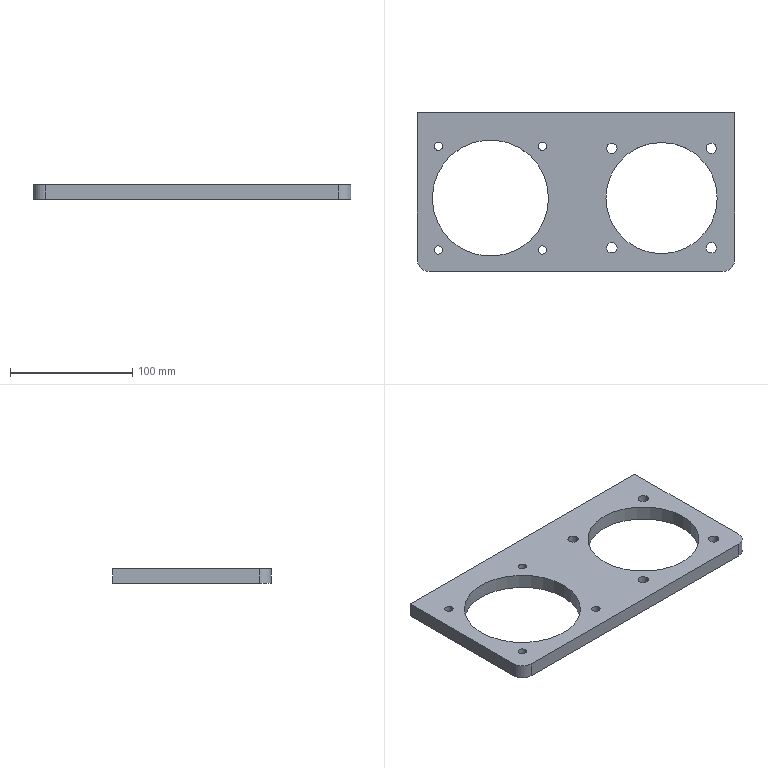Part | SolidWorks | features HoleWzd 2, FlatPattern 1, SMBaseFlange 1, SheetMetal 1 | 1 solid | 28 faces | box 260 x 130 x 12 mm | volume 237513 mm3 | cylinder 22 | plane 6 | commonest cylinder face diameters 6.8 x8 8.5 x8 20 x2 91 x2 95 x2
STEP:
#1=CARTESIAN_POINT('',(25.1,35.65,-12.));
#2=VERTEX_POINT('',#1);
#3=CARTESIAN_POINT('',(33.6,35.65,-12.));
#4=VERTEX_POINT('',#3);
#5=CARTESIAN_POINT('',(29.35,35.65,-12.));
#6=DIRECTION('',(0.,0.,1.));
#7=DIRECTION('',(1.,0.,0.));
#8=AXIS2_PLACEMENT_3D('',#5,#6,#7);
#9=CIRCLE('',#8,4.25);
#10=EDGE_CURVE('',#2,#4,#9,.T.);
#11=ORIENTED_EDGE('',*,*,#10,.F.);
#12=CARTESIAN_POINT('',(25.1,35.65,0.));
#13=VERTEX_POINT('',#12);
#14=CARTESIAN_POINT('',(25.1,35.65,0.));
#15=DIRECTION('',(0.,0.,1.));
#16=VECTOR('',#15,1000.);
#17=LINE('',#14,#16);
#18=EDGE_CURVE('',#2,#13,#17,.T.);
#19=ORIENTED_EDGE('',*,*,#18,.T.);
#20=CARTESIAN_POINT('',(33.6,35.65,0.));
#21=VERTEX_POINT('',#20);
#22=CARTESIAN_POINT('',(29.35,35.65,0.));
#23=DIRECTION('',(0.,0.,1.));
#24=DIRECTION('',(1.,0.,0.));
#25=AXIS2_PLACEMENT_3D('',#22,#23,#24);
#26=CIRCLE('',#25,4.25);
#27=EDGE_CURVE('',#13,#21,#26,.T.);
#28=ORIENTED_EDGE('',*,*,#27,.T.);
#29=CARTESIAN_POINT('',(33.6,35.65,0.));
#30=DIRECTION('',(0.,0.,1.));
#31=VECTOR('',#30,1000.);
#32=LINE('',#29,#31);
#33=EDGE_CURVE('',#4,#21,#32,.T.);
#34=ORIENTED_EDGE('',*,*,#33,.F.);
#35=EDGE_LOOP('',(#11,#19,#28,#34));
#36=FACE_OUTER_BOUND('',#35,.T.);
#37=CARTESIAN_POINT('',(29.35,35.65,0.));
#38=DIRECTION('',(0.,0.,1.));
#39=DIRECTION('',(1.,0.,0.));
#40=AXIS2_PLACEMENT_3D('',#37,#38,#39);
#41=CYLINDRICAL_SURFACE('',#40,4.25);
#42=ADVANCED_FACE('',(#36),#41,.F.);
#43=CARTESIAN_POINT('',(106.4,35.65,-12.));
#44=VERTEX_POINT('',#43);
#45=CARTESIAN_POINT('',(114.9,35.65,-12.));
#46=VERTEX_POINT('',#45);
#47=CARTESIAN_POINT('',(110.65,35.65,-12.));
#48=DIRECTION('',(0.,0.,1.));
#49=DIRECTION('',(1.,0.,0.));
#50=AXIS2_PLACEMENT_3D('',#47,#48,#49);
#51=CIRCLE('',#50,4.25);
#52=EDGE_CURVE('',#44,#46,#51,.T.);
#53=ORIENTED_EDGE('',*,*,#52,.F.);
#54=CARTESIAN_POINT('',(106.4,35.65,0.));
#55=VERTEX_POINT('',#54);
#56=CARTESIAN_POINT('',(106.4,35.65,0.));
#57=DIRECTION('',(0.,0.,1.));
#58=VECTOR('',#57,1000.);
#59=LINE('',#56,#58);
#60=EDGE_CURVE('',#44,#55,#59,.T.);
#61=ORIENTED_EDGE('',*,*,#60,.T.);
#62=CARTESIAN_POINT('',(114.9,35.65,0.));
#63=VERTEX_POINT('',#62);
#64=CARTESIAN_POINT('',(110.65,35.65,0.));
#65=DIRECTION('',(0.,0.,1.));
#66=DIRECTION('',(1.,0.,0.));
#67=AXIS2_PLACEMENT_3D('',#64,#65,#66);
#68=CIRCLE('',#67,4.25);
#69=EDGE_CURVE('',#55,#63,#68,.T.);
#70=ORIENTED_EDGE('',*,*,#69,.T.);
#71=CARTESIAN_POINT('',(114.9,35.65,0.));
#72=DIRECTION('',(0.,0.,1.));
#73=VECTOR('',#72,1000.);
#74=LINE('',#71,#73);
#75=EDGE_CURVE('',#46,#63,#74,.T.);
#76=ORIENTED_EDGE('',*,*,#75,.F.);
#77=EDGE_LOOP('',(#53,#61,#70,#76));
#78=FACE_OUTER_BOUND('',#77,.T.);
#79=CARTESIAN_POINT('',(110.65,35.65,0.));
#80=DIRECTION('',(0.,0.,1.));
#81=DIRECTION('',(1.,0.,0.));
#82=AXIS2_PLACEMENT_3D('',#79,#80,#81);
#83=CYLINDRICAL_SURFACE('',#82,4.25);
#84=ADVANCED_FACE('',(#78),#83,.F.);
#85=CARTESIAN_POINT('',(106.4,-45.65,-12.));
#86=VERTEX_POINT('',#85);
#87=CARTESIAN_POINT('',(114.9,-45.65,-12.));
#88=VERTEX_POINT('',#87);
#89=CARTESIAN_POINT('',(110.65,-45.65,-12.));
#90=DIRECTION('',(0.,0.,1.));
#91=DIRECTION('',(1.,0.,0.));
#92=AXIS2_PLACEMENT_3D('',#89,#90,#91);
#93=CIRCLE('',#92,4.25);
#94=EDGE_CURVE('',#86,#88,#93,.T.);
#95=ORIENTED_EDGE('',*,*,#94,.F.);
#96=CARTESIAN_POINT('',(106.4,-45.65,0.));
#97=VERTEX_POINT('',#96);
#98=CARTESIAN_POINT('',(106.4,-45.65,0.));
#99=DIRECTION('',(0.,0.,1.));
#100=VECTOR('',#99,1000.);
#101=LINE('',#98,#100);
#102=EDGE_CURVE('',#86,#97,#101,.T.);
#103=ORIENTED_EDGE('',*,*,#102,.T.);
#104=CARTESIAN_POINT('',(114.9,-45.65,0.));
#105=VERTEX_POINT('',#104);
#106=CARTESIAN_POINT('',(110.65,-45.65,0.));
#107=DIRECTION('',(0.,0.,1.));
#108=DIRECTION('',(1.,0.,0.));
#109=AXIS2_PLACEMENT_3D('',#106,#107,#108);
#110=CIRCLE('',#109,4.25);
#111=EDGE_CURVE('',#97,#105,#110,.T.);
#112=ORIENTED_EDGE('',*,*,#111,.T.);
#113=CARTESIAN_POINT('',(114.9,-45.65,0.));
#114=DIRECTION('',(0.,0.,1.));
#115=VECTOR('',#114,1000.);
#116=LINE('',#113,#115);
#117=EDGE_CURVE('',#88,#105,#116,.T.);
#118=ORIENTED_EDGE('',*,*,#117,.F.);
#119=EDGE_LOOP('',(#95,#103,#112,#118));
#120=FACE_OUTER_BOUND('',#119,.T.);
#121=CARTESIAN_POINT('',(110.65,-45.65,0.));
#122=DIRECTION('',(0.,0.,1.));
#123=DIRECTION('',(1.,0.,0.));
#124=AXIS2_PLACEMENT_3D('',#121,#122,#123);
#125=CYLINDRICAL_SURFACE('',#124,4.25);
#126=ADVANCED_FACE('',(#120),#125,.F.);
#127=CARTESIAN_POINT('',(25.1,-45.65,-12.));
#128=VERTEX_POINT('',#127);
#129=CARTESIAN_POINT('',(33.6,-45.65,-12.));
#130=VERTEX_POINT('',#129);
#131=CARTESIAN_POINT('',(29.35,-45.65,-12.));
#132=DIRECTION('',(0.,0.,1.));
#133=DIRECTION('',(1.,0.,0.));
#134=AXIS2_PLACEMENT_3D('',#131,#132,#133);
#135=CIRCLE('',#134,4.25);
#136=EDGE_CURVE('',#128,#130,#135,.T.);
#137=ORIENTED_EDGE('',*,*,#136,.F.);
#138=CARTESIAN_POINT('',(25.1,-45.65,0.));
#139=VERTEX_POINT('',#138);
#140=CARTESIAN_POINT('',(25.1,-45.65,0.));
#141=DIRECTION('',(0.,0.,1.));
#142=VECTOR('',#141,1000.);
#143=LINE('',#140,#142);
#144=EDGE_CURVE('',#128,#139,#143,.T.);
#145=ORIENTED_EDGE('',*,*,#144,.T.);
#146=CARTESIAN_POINT('',(33.6,-45.65,0.));
#147=VERTEX_POINT('',#146);
#148=CARTESIAN_POINT('',(29.35,-45.65,0.));
#149=DIRECTION('',(0.,0.,1.));
#150=DIRECTION('',(1.,0.,0.));
#151=AXIS2_PLACEMENT_3D('',#148,#149,#150);
#152=CIRCLE('',#151,4.25);
#153=EDGE_CURVE('',#139,#147,#152,.T.);
#154=ORIENTED_EDGE('',*,*,#153,.T.);
#155=CARTESIAN_POINT('',(33.6,-45.65,0.));
#156=DIRECTION('',(0.,0.,1.));
#157=VECTOR('',#156,1000.);
#158=LINE('',#155,#157);
#159=EDGE_CURVE('',#130,#147,#158,.T.);
#160=ORIENTED_EDGE('',*,*,#159,.F.);
#161=EDGE_LOOP('',(#137,#145,#154,#160));
#162=FACE_OUTER_BOUND('',#161,.T.);
#163=CARTESIAN_POINT('',(29.35,-45.65,0.));
#164=DIRECTION('',(0.,0.,1.));
#165=DIRECTION('',(1.,0.,0.));
#166=AXIS2_PLACEMENT_3D('',#163,#164,#165);
#167=CYLINDRICAL_SURFACE('',#166,4.25);
#168=ADVANCED_FACE('',(#162),#167,.F.);
#169=CARTESIAN_POINT('',(-115.9,37.5,-12.));
#170=VERTEX_POINT('',#169);
#171=CARTESIAN_POINT('',(-109.1,37.5,-12.));
#172=VERTEX_POINT('',#171);
#173=CARTESIAN_POINT('',(-112.5,37.5,-12.));
#174=DIRECTION('',(0.,0.,1.));
#175=DIRECTION('',(1.,0.,0.));
#176=AXIS2_PLACEMENT_3D('',#173,#174,#175);
#177=CIRCLE('',#176,3.4);
#178=EDGE_CURVE('',#170,#172,#177,.T.);
#179=ORIENTED_EDGE('',*,*,#178,.F.);
#180=CARTESIAN_POINT('',(-115.9,37.5,0.));
#181=VERTEX_POINT('',#180);
#182=CARTESIAN_POINT('',(-115.9,37.5,0.));
#183=DIRECTION('',(0.,0.,1.));
#184=VECTOR('',#183,1000.);
#185=LINE('',#182,#184);
#186=EDGE_CURVE('',#170,#181,#185,.T.);
#187=ORIENTED_EDGE('',*,*,#186,.T.);
#188=CARTESIAN_POINT('',(-109.1,37.5,0.));
#189=VERTEX_POINT('',#188);
#190=CARTESIAN_POINT('',(-112.5,37.5,0.));
#191=DIRECTION('',(0.,0.,1.));
#192=DIRECTION('',(1.,0.,0.));
#193=AXIS2_PLACEMENT_3D('',#190,#191,#192);
#194=CIRCLE('',#193,3.4);
#195=EDGE_CURVE('',#181,#189,#194,.T.);
#196=ORIENTED_EDGE('',*,*,#195,.T.);
#197=CARTESIAN_POINT('',(-109.1,37.5,0.));
#198=DIRECTION('',(0.,0.,1.));
#199=VECTOR('',#198,1000.);
#200=LINE('',#197,#199);
#201=EDGE_CURVE('',#172,#189,#200,.T.);
#202=ORIENTED_EDGE('',*,*,#201,.F.);
#203=EDGE_LOOP('',(#179,#187,#196,#202));
#204=FACE_OUTER_BOUND('',#203,.T.);
#205=CARTESIAN_POINT('',(-112.5,37.5,0.));
#206=DIRECTION('',(0.,0.,1.));
#207=DIRECTION('',(1.,0.,0.));
#208=AXIS2_PLACEMENT_3D('',#205,#206,#207);
#209=CYLINDRICAL_SURFACE('',#208,3.4);
#210=ADVANCED_FACE('',(#204),#209,.F.);
#211=CARTESIAN_POINT('',(-30.9,37.5,-12.));
#212=VERTEX_POINT('',#211);
#213=CARTESIAN_POINT('',(-24.1,37.5,-12.));
#214=VERTEX_POINT('',#213);
#215=CARTESIAN_POINT('',(-27.5,37.5,-12.));
#216=DIRECTION('',(0.,0.,1.));
#217=DIRECTION('',(1.,0.,0.));
#218=AXIS2_PLACEMENT_3D('',#215,#216,#217);
#219=CIRCLE('',#218,3.4);
#220=EDGE_CURVE('',#212,#214,#219,.T.);
#221=ORIENTED_EDGE('',*,*,#220,.F.);
#222=CARTESIAN_POINT('',(-30.9,37.5,0.));
#223=VERTEX_POINT('',#222);
#224=CARTESIAN_POINT('',(-30.9,37.5,0.));
#225=DIRECTION('',(0.,0.,1.));
#226=VECTOR('',#225,1000.);
#227=LINE('',#224,#226);
#228=EDGE_CURVE('',#212,#223,#227,.T.);
#229=ORIENTED_EDGE('',*,*,#228,.T.);
#230=CARTESIAN_POINT('',(-24.1,37.5,0.));
#231=VERTEX_POINT('',#230);
#232=CARTESIAN_POINT('',(-27.5,37.5,0.));
#233=DIRECTION('',(0.,0.,1.));
#234=DIRECTION('',(1.,0.,0.));
#235=AXIS2_PLACEMENT_3D('',#232,#233,#234);
#236=CIRCLE('',#235,3.4);
#237=EDGE_CURVE('',#223,#231,#236,.T.);
#238=ORIENTED_EDGE('',*,*,#237,.T.);
#239=CARTESIAN_POINT('',(-24.1,37.5,0.));
#240=DIRECTION('',(0.,0.,1.));
#241=VECTOR('',#240,1000.);
#242=LINE('',#239,#241);
#243=EDGE_CURVE('',#214,#231,#242,.T.);
#244=ORIENTED_EDGE('',*,*,#243,.F.);
#245=EDGE_LOOP('',(#221,#229,#238,#244));
#246=FACE_OUTER_BOUND('',#245,.T.);
#247=CARTESIAN_POINT('',(-27.5,37.5,0.));
#248=DIRECTION('',(0.,0.,1.));
#249=DIRECTION('',(1.,0.,0.));
#250=AXIS2_PLACEMENT_3D('',#247,#248,#249);
#251=CYLINDRICAL_SURFACE('',#250,3.4);
#252=ADVANCED_FACE('',(#246),#251,.F.);
#253=CARTESIAN_POINT('',(-30.9,-47.5,-12.));
#254=VERTEX_POINT('',#253);
#255=CARTESIAN_POINT('',(-24.1,-47.5,-12.));
#256=VERTEX_POINT('',#255);
#257=CARTESIAN_POINT('',(-27.5,-47.5,-12.));
#258=DIRECTION('',(0.,0.,1.));
#259=DIRECTION('',(1.,0.,0.));
#260=AXIS2_PLACEMENT_3D('',#257,#258,#259);
#261=CIRCLE('',#260,3.4);
#262=EDGE_CURVE('',#254,#256,#261,.T.);
#263=ORIENTED_EDGE('',*,*,#262,.F.);
#264=CARTESIAN_POINT('',(-30.9,-47.5,0.));
#265=VERTEX_POINT('',#264);
#266=CARTESIAN_POINT('',(-30.9,-47.5,0.));
#267=DIRECTION('',(0.,0.,1.));
#268=VECTOR('',#267,1000.);
#269=LINE('',#266,#268);
#270=EDGE_CURVE('',#254,#265,#269,.T.);
#271=ORIENTED_EDGE('',*,*,#270,.T.);
#272=CARTESIAN_POINT('',(-24.1,-47.5,0.));
#273=VERTEX_POINT('',#272);
#274=CARTESIAN_POINT('',(-27.5,-47.5,0.));
#275=DIRECTION('',(0.,0.,1.));
#276=DIRECTION('',(1.,0.,0.));
#277=AXIS2_PLACEMENT_3D('',#274,#275,#276);
#278=CIRCLE('',#277,3.4);
#279=EDGE_CURVE('',#265,#273,#278,.T.);
#280=ORIENTED_EDGE('',*,*,#279,.T.);
#281=CARTESIAN_POINT('',(-24.1,-47.5,0.));
#282=DIRECTION('',(0.,0.,1.));
#283=VECTOR('',#282,1000.);
#284=LINE('',#281,#283);
#285=EDGE_CURVE('',#256,#273,#284,.T.);
#286=ORIENTED_EDGE('',*,*,#285,.F.);
#287=EDGE_LOOP('',(#263,#271,#280,#286));
#288=FACE_OUTER_BOUND('',#287,.T.);
#289=CARTESIAN_POINT('',(-27.5,-47.5,0.));
#290=DIRECTION('',(0.,0.,1.));
#291=DIRECTION('',(1.,0.,0.));
#292=AXIS2_PLACEMENT_3D('',#289,#290,#291);
#293=CYLINDRICAL_SURFACE('',#292,3.4);
#294=ADVANCED_FACE('',(#288),#293,.F.);
#295=CARTESIAN_POINT('',(-115.9,-47.5,-12.));
#296=VERTEX_POINT('',#295);
#297=CARTESIAN_POINT('',(-109.1,-47.5,-12.));
#298=VERTEX_POINT('',#297);
#299=CARTESIAN_POINT('',(-112.5,-47.5,-12.));
#300=DIRECTION('',(0.,0.,1.));
#301=DIRECTION('',(1.,0.,0.));
#302=AXIS2_PLACEMENT_3D('',#299,#300,#301);
#303=CIRCLE('',#302,3.4);
#304=EDGE_CURVE('',#296,#298,#303,.T.);
#305=ORIENTED_EDGE('',*,*,#304,.F.);
#306=CARTESIAN_POINT('',(-115.9,-47.5,0.));
#307=VERTEX_POINT('',#306);
#308=CARTESIAN_POINT('',(-115.9,-47.5,0.));
#309=DIRECTION('',(0.,0.,1.));
#310=VECTOR('',#309,1000.);
#311=LINE('',#308,#310);
#312=EDGE_CURVE('',#296,#307,#311,.T.);
#313=ORIENTED_EDGE('',*,*,#312,.T.);
#314=CARTESIAN_POINT('',(-109.1,-47.5,0.));
#315=VERTEX_POINT('',#314);
#316=CARTESIAN_POINT('',(-112.5,-47.5,0.));
#317=DIRECTION('',(0.,0.,1.));
#318=DIRECTION('',(1.,0.,0.));
#319=AXIS2_PLACEMENT_3D('',#316,#317,#318);
#320=CIRCLE('',#319,3.4);
#321=EDGE_CURVE('',#307,#315,#320,.T.);
#322=ORIENTED_EDGE('',*,*,#321,.T.);
#323=CARTESIAN_POINT('',(-109.1,-47.5,0.));
#324=DIRECTION('',(0.,0.,1.));
#325=VECTOR('',#324,1000.);
#326=LINE('',#323,#325);
#327=EDGE_CURVE('',#298,#315,#326,.T.);
#328=ORIENTED_EDGE('',*,*,#327,.F.);
#329=EDGE_LOOP('',(#305,#313,#322,#328));
#330=FACE_OUTER_BOUND('',#329,.T.);
#331=CARTESIAN_POINT('',(-112.5,-47.5,0.));
#332=DIRECTION('',(0.,0.,1.));
#333=DIRECTION('',(1.,0.,0.));
#334=AXIS2_PLACEMENT_3D('',#331,#332,#333);
#335=CYLINDRICAL_SURFACE('',#334,3.4);
#336=ADVANCED_FACE('',(#330),#335,.F.);
#337=CARTESIAN_POINT('',(24.5,-5.,-12.));
#338=VERTEX_POINT('',#337);
#339=CARTESIAN_POINT('',(115.5,-5.,-12.));
#340=VERTEX_POINT('',#339);
#341=CARTESIAN_POINT('',(70.,-5.,-12.));
#342=DIRECTION('',(0.,0.,1.));
#343=DIRECTION('',(1.,0.,0.));
#344=AXIS2_PLACEMENT_3D('',#341,#342,#343);
#345=CIRCLE('',#344,45.5);
#346=EDGE_CURVE('',#338,#340,#345,.T.);
#347=ORIENTED_EDGE('',*,*,#346,.F.);
#348=CARTESIAN_POINT('',(24.5,-5.,0.));
#349=VERTEX_POINT('',#348);
#350=CARTESIAN_POINT('',(24.5,-5.,-12.));
#351=DIRECTION('',(0.,0.,1.));
#352=VECTOR('',#351,1000.);
#353=LINE('',#350,#352);
#354=EDGE_CURVE('',#338,#349,#353,.T.);
#355=ORIENTED_EDGE('',*,*,#354,.T.);
#356=CARTESIAN_POINT('',(115.5,-5.,0.));
#357=VERTEX_POINT('',#356);
#358=CARTESIAN_POINT('',(70.,-5.,0.));
#359=DIRECTION('',(0.,0.,1.));
#360=DIRECTION('',(1.,0.,0.));
#361=AXIS2_PLACEMENT_3D('',#358,#359,#360);
#362=CIRCLE('',#361,45.5);
#363=EDGE_CURVE('',#349,#357,#362,.T.);
#364=ORIENTED_EDGE('',*,*,#363,.T.);
#365=CARTESIAN_POINT('',(115.5,-5.,-12.));
#366=DIRECTION('',(0.,0.,1.));
#367=VECTOR('',#366,1000.);
#368=LINE('',#365,#367);
#369=EDGE_CURVE('',#340,#357,#368,.T.);
#370=ORIENTED_EDGE('',*,*,#369,.F.);
#371=EDGE_LOOP('',(#347,#355,#364,#370));
#372=FACE_OUTER_BOUND('',#371,.T.);
#373=CARTESIAN_POINT('',(70.,-5.,-12.));
#374=DIRECTION('',(0.,0.,1.));
#375=DIRECTION('',(1.,0.,0.));
#376=AXIS2_PLACEMENT_3D('',#373,#374,#375);
#377=CYLINDRICAL_SURFACE('',#376,45.5);
#378=ADVANCED_FACE('',(#372),#377,.F.);
#379=CARTESIAN_POINT('',(-117.5,-5.,-12.));
#380=VERTEX_POINT('',#379);
#381=CARTESIAN_POINT('',(-22.5,-5.,-12.));
#382=VERTEX_POINT('',#381);
#383=CARTESIAN_POINT('',(-70.,-5.,-12.));
#384=DIRECTION('',(0.,0.,1.));
#385=DIRECTION('',(1.,0.,0.));
#386=AXIS2_PLACEMENT_3D('',#383,#384,#385);
#387=CIRCLE('',#386,47.5);
#388=EDGE_CURVE('',#380,#382,#387,.T.);
#389=ORIENTED_EDGE('',*,*,#388,.F.);
#390=CARTESIAN_POINT('',(-117.5,-5.,0.));
#391=VERTEX_POINT('',#390);
#392=CARTESIAN_POINT('',(-117.5,-5.,-12.));
#393=DIRECTION('',(0.,0.,1.));
#394=VECTOR('',#393,1000.);
#395=LINE('',#392,#394);
#396=EDGE_CURVE('',#380,#391,#395,.T.);
#397=ORIENTED_EDGE('',*,*,#396,.T.);
#398=CARTESIAN_POINT('',(-22.5,-5.,0.));
#399=VERTEX_POINT('',#398);
#400=CARTESIAN_POINT('',(-70.,-5.,0.));
#401=DIRECTION('',(0.,0.,1.));
#402=DIRECTION('',(1.,0.,0.));
#403=AXIS2_PLACEMENT_3D('',#400,#401,#402);
#404=CIRCLE('',#403,47.5);
#405=EDGE_CURVE('',#391,#399,#404,.T.);
#406=ORIENTED_EDGE('',*,*,#405,.T.);
#407=CARTESIAN_POINT('',(-22.5,-5.,-12.));
#408=DIRECTION('',(0.,0.,1.));
#409=VECTOR('',#408,1000.);
#410=LINE('',#407,#409);
#411=EDGE_CURVE('',#382,#399,#410,.T.);
#412=ORIENTED_EDGE('',*,*,#411,.F.);
#413=EDGE_LOOP('',(#389,#397,#406,#412));
#414=FACE_OUTER_BOUND('',#413,.T.);
#415=CARTESIAN_POINT('',(-70.,-5.,-12.));
#416=DIRECTION('',(0.,0.,1.));
#417=DIRECTION('',(1.,0.,0.));
#418=AXIS2_PLACEMENT_3D('',#415,#416,#417);
#419=CYLINDRICAL_SURFACE('',#418,47.5);
#420=ADVANCED_FACE('',(#414),#419,.F.);
#421=CARTESIAN_POINT('',(-130.,65.,0.));
#422=VERTEX_POINT('',#421);
#423=CARTESIAN_POINT('',(-130.,-55.,0.));
#424=VERTEX_POINT('',#423);
#425=CARTESIAN_POINT('',(-130.,65.,0.));
#426=DIRECTION('',(0.,-1.,0.));
#427=VECTOR('',#426,1000.);
#428=LINE('',#425,#427);
#429=EDGE_CURVE('',#422,#424,#428,.T.);
#430=ORIENTED_EDGE('',*,*,#429,.F.);
#431=CARTESIAN_POINT('',(-130.,65.,-12.));
#432=VERTEX_POINT('',#431);
#433=CARTESIAN_POINT('',(-130.,65.,-12.));
#434=DIRECTION('',(0.,0.,1.));
#435=VECTOR('',#434,1000.);
#436=LINE('',#433,#435);
#437=EDGE_CURVE('',#432,#422,#436,.T.);
#438=ORIENTED_EDGE('',*,*,#437,.F.);
#439=CARTESIAN_POINT('',(-130.,-55.,-12.));
#440=VERTEX_POINT('',#439);
#441=CARTESIAN_POINT('',(-130.,65.,-12.));
#442=DIRECTION('',(0.,-1.,0.));
#443=VECTOR('',#442,1000.);
#444=LINE('',#441,#443);
#445=EDGE_CURVE('',#432,#440,#444,.T.);
#446=ORIENTED_EDGE('',*,*,#445,.T.);
#447=CARTESIAN_POINT('',(-130.,-55.,-12.));
#448=DIRECTION('',(0.,0.,1.));
#449=VECTOR('',#448,1000.);
#450=LINE('',#447,#449);
#451=EDGE_CURVE('',#440,#424,#450,.T.);
#452=ORIENTED_EDGE('',*,*,#451,.T.);
#453=EDGE_LOOP('',(#430,#438,#446,#452));
#454=FACE_OUTER_BOUND('',#453,.T.);
#455=CARTESIAN_POINT('',(-130.,65.,-12.));
#456=DIRECTION('',(-1.,0.,0.));
#457=DIRECTION('',(0.,-1.,0.));
#458=AXIS2_PLACEMENT_3D('',#455,#456,#457);
#459=PLANE('',#458);
#460=ADVANCED_FACE('',(#454),#459,.T.);
#461=CARTESIAN_POINT('',(130.,65.,0.));
#462=VERTEX_POINT('',#461);
#463=CARTESIAN_POINT('',(-130.,65.,0.));
#464=DIRECTION('',(-1.,0.,0.));
#465=VECTOR('',#464,1000.);
#466=LINE('',#463,#465);
#467=EDGE_CURVE('',#462,#422,#466,.T.);
#468=ORIENTED_EDGE('',*,*,#467,.F.);
#469=CARTESIAN_POINT('',(130.,65.,-12.));
#470=VERTEX_POINT('',#469);
#471=CARTESIAN_POINT('',(130.,65.,-12.));
#472=DIRECTION('',(0.,0.,1.));
#473=VECTOR('',#472,1000.);
#474=LINE('',#471,#473);
#475=EDGE_CURVE('',#470,#462,#474,.T.);
#476=ORIENTED_EDGE('',*,*,#475,.F.);
#477=CARTESIAN_POINT('',(-130.,65.,-12.));
#478=DIRECTION('',(-1.,0.,0.));
#479=VECTOR('',#478,1000.);
#480=LINE('',#477,#479);
#481=EDGE_CURVE('',#470,#432,#480,.T.);
#482=ORIENTED_EDGE('',*,*,#481,.T.);
#483=ORIENTED_EDGE('',*,*,#437,.T.);
#484=EDGE_LOOP('',(#468,#476,#482,#483));
#485=FACE_OUTER_BOUND('',#484,.T.);
#486=CARTESIAN_POINT('',(-130.,65.,-12.));
#487=DIRECTION('',(0.,1.,0.));
#488=DIRECTION('',(0.,0.,1.));
#489=AXIS2_PLACEMENT_3D('',#486,#487,#488);
#490=PLANE('',#489);
#491=ADVANCED_FACE('',(#485),#490,.T.);
#492=CARTESIAN_POINT('',(130.,-55.,0.));
#493=VERTEX_POINT('',#492);
#494=CARTESIAN_POINT('',(130.,65.,0.));
#495=DIRECTION('',(0.,1.,0.));
#496=VECTOR('',#495,1000.);
#497=LINE('',#494,#496);
#498=EDGE_CURVE('',#493,#462,#497,.T.);
#499=ORIENTED_EDGE('',*,*,#498,.F.);
#500=CARTESIAN_POINT('',(130.,-55.,-12.));
#501=VERTEX_POINT('',#500);
#502=CARTESIAN_POINT('',(130.,-55.,-12.));
#503=DIRECTION('',(0.,0.,1.));
#504=VECTOR('',#503,1000.);
#505=LINE('',#502,#504);
#506=EDGE_CURVE('',#501,#493,#505,.T.);
#507=ORIENTED_EDGE('',*,*,#506,.F.);
#508=CARTESIAN_POINT('',(130.,65.,-12.));
#509=DIRECTION('',(0.,1.,0.));
#510=VECTOR('',#509,1000.);
#511=LINE('',#508,#510);
#512=EDGE_CURVE('',#501,#470,#511,.T.);
#513=ORIENTED_EDGE('',*,*,#512,.T.);
#514=ORIENTED_EDGE('',*,*,#475,.T.);
#515=EDGE_LOOP('',(#499,#507,#513,#514));
#516=FACE_OUTER_BOUND('',#515,.T.);
#517=CARTESIAN_POINT('',(130.,65.,-12.));
#518=DIRECTION('',(1.,0.,0.));
#519=DIRECTION('',(0.,1.,0.));
#520=AXIS2_PLACEMENT_3D('',#517,#518,#519);
#521=PLANE('',#520);
#522=ADVANCED_FACE('',(#516),#521,.T.);
#523=CARTESIAN_POINT('',(120.,-65.,0.));
#524=VERTEX_POINT('',#523);
#525=CARTESIAN_POINT('',(120.,-55.,0.));
#526=DIRECTION('',(0.,0.,1.));
#527=DIRECTION('',(1.,0.,0.));
#528=AXIS2_PLACEMENT_3D('',#525,#526,#527);
#529=CIRCLE('',#528,10.);
#530=EDGE_CURVE('',#524,#493,#529,.T.);
#531=ORIENTED_EDGE('',*,*,#530,.F.);
#532=CARTESIAN_POINT('',(120.,-65.,-12.));
#533=VERTEX_POINT('',#532);
#534=CARTESIAN_POINT('',(120.,-65.,-12.));
#535=DIRECTION('',(0.,0.,1.));
#536=VECTOR('',#535,1000.);
#537=LINE('',#534,#536);
#538=EDGE_CURVE('',#533,#524,#537,.T.);
#539=ORIENTED_EDGE('',*,*,#538,.F.);
#540=CARTESIAN_POINT('',(120.,-55.,-12.));
#541=DIRECTION('',(0.,0.,1.));
#542=DIRECTION('',(1.,0.,0.));
#543=AXIS2_PLACEMENT_3D('',#540,#541,#542);
#544=CIRCLE('',#543,10.);
#545=EDGE_CURVE('',#533,#501,#544,.T.);
#546=ORIENTED_EDGE('',*,*,#545,.T.);
#547=ORIENTED_EDGE('',*,*,#506,.T.);
#548=EDGE_LOOP('',(#531,#539,#546,#547));
#549=FACE_OUTER_BOUND('',#548,.T.);
#550=CARTESIAN_POINT('',(120.,-55.,-12.));
#551=DIRECTION('',(0.,0.,1.));
#552=DIRECTION('',(1.,0.,0.));
#553=AXIS2_PLACEMENT_3D('',#550,#551,#552);
#554=CYLINDRICAL_SURFACE('',#553,10.);
#555=ADVANCED_FACE('',(#549),#554,.T.);
#556=CARTESIAN_POINT('',(-120.,-65.,0.));
#557=VERTEX_POINT('',#556);
#558=CARTESIAN_POINT('',(-120.,-65.,0.));
#559=DIRECTION('',(1.,0.,0.));
#560=VECTOR('',#559,1000.);
#561=LINE('',#558,#560);
#562=EDGE_CURVE('',#557,#524,#561,.T.);
#563=ORIENTED_EDGE('',*,*,#562,.F.);
#564=CARTESIAN_POINT('',(-120.,-65.,-12.));
#565=VERTEX_POINT('',#564);
#566=CARTESIAN_POINT('',(-120.,-65.,-12.));
#567=DIRECTION('',(0.,0.,1.));
#568=VECTOR('',#567,1000.);
#569=LINE('',#566,#568);
#570=EDGE_CURVE('',#565,#557,#569,.T.);
#571=ORIENTED_EDGE('',*,*,#570,.F.);
#572=CARTESIAN_POINT('',(-120.,-65.,-12.));
#573=DIRECTION('',(1.,0.,0.));
#574=VECTOR('',#573,1000.);
#575=LINE('',#572,#574);
#576=EDGE_CURVE('',#565,#533,#575,.T.);
#577=ORIENTED_EDGE('',*,*,#576,.T.);
#578=ORIENTED_EDGE('',*,*,#538,.T.);
#579=EDGE_LOOP('',(#563,#571,#577,#578));
#580=FACE_OUTER_BOUND('',#579,.T.);
#581=CARTESIAN_POINT('',(-120.,-65.,-12.));
#582=DIRECTION('',(0.,-1.,0.));
#583=DIRECTION('',(0.,0.,-1.));
#584=AXIS2_PLACEMENT_3D('',#581,#582,#583);
#585=PLANE('',#584);
#586=ADVANCED_FACE('',(#580),#585,.T.);
#587=CARTESIAN_POINT('',(-120.,-55.,0.));
#588=DIRECTION('',(0.,0.,1.));
#589=DIRECTION('',(1.,0.,0.));
#590=AXIS2_PLACEMENT_3D('',#587,#588,#589);
#591=CIRCLE('',#590,10.);
#592=EDGE_CURVE('',#424,#557,#591,.T.);
#593=ORIENTED_EDGE('',*,*,#592,.F.);
#594=ORIENTED_EDGE('',*,*,#451,.F.);
#595=CARTESIAN_POINT('',(-120.,-55.,-12.));
#596=DIRECTION('',(0.,0.,1.));
#597=DIRECTION('',(1.,0.,0.));
#598=AXIS2_PLACEMENT_3D('',#595,#596,#597);
#599=CIRCLE('',#598,10.);
#600=EDGE_CURVE('',#440,#565,#599,.T.);
#601=ORIENTED_EDGE('',*,*,#600,.T.);
#602=ORIENTED_EDGE('',*,*,#570,.T.);
#603=EDGE_LOOP('',(#593,#594,#601,#602));
#604=FACE_OUTER_BOUND('',#603,.T.);
#605=CARTESIAN_POINT('',(-120.,-55.,-12.));
#606=DIRECTION('',(0.,0.,1.));
#607=DIRECTION('',(1.,0.,0.));
#608=AXIS2_PLACEMENT_3D('',#605,#606,#607);
#609=CYLINDRICAL_SURFACE('',#608,10.);
#610=ADVANCED_FACE('',(#604),#609,.T.);
#611=CARTESIAN_POINT('',(29.35,35.65,-12.));
#612=DIRECTION('',(0.,0.,1.));
#613=DIRECTION('',(1.,0.,0.));
#614=AXIS2_PLACEMENT_3D('',#611,#612,#613);
#615=CIRCLE('',#614,4.25);
#616=EDGE_CURVE('',#4,#2,#615,.T.);
#617=ORIENTED_EDGE('',*,*,#616,.T.);
#618=ORIENTED_EDGE('',*,*,#10,.T.);
#619=EDGE_LOOP('',(#617,#618));
#620=FACE_BOUND('',#619,.T.);
#621=CARTESIAN_POINT('',(110.65,35.65,-12.));
#622=DIRECTION('',(0.,0.,1.));
#623=DIRECTION('',(1.,0.,0.));
#624=AXIS2_PLACEMENT_3D('',#621,#622,#623);
#625=CIRCLE('',#624,4.25);
#626=EDGE_CURVE('',#46,#44,#625,.T.);
#627=ORIENTED_EDGE('',*,*,#626,.T.);
#628=ORIENTED_EDGE('',*,*,#52,.T.);
#629=EDGE_LOOP('',(#627,#628));
#630=FACE_BOUND('',#629,.T.);
#631=CARTESIAN_POINT('',(110.65,-45.65,-12.));
#632=DIRECTION('',(0.,0.,1.));
#633=DIRECTION('',(1.,0.,0.));
#634=AXIS2_PLACEMENT_3D('',#631,#632,#633);
#635=CIRCLE('',#634,4.25);
#636=EDGE_CURVE('',#88,#86,#635,.T.);
#637=ORIENTED_EDGE('',*,*,#636,.T.);
#638=ORIENTED_EDGE('',*,*,#94,.T.);
#639=EDGE_LOOP('',(#637,#638));
#640=FACE_BOUND('',#639,.T.);
#641=CARTESIAN_POINT('',(29.35,-45.65,-12.));
#642=DIRECTION('',(0.,0.,1.));
#643=DIRECTION('',(1.,0.,0.));
#644=AXIS2_PLACEMENT_3D('',#641,#642,#643);
#645=CIRCLE('',#644,4.25);
#646=EDGE_CURVE('',#130,#128,#645,.T.);
#647=ORIENTED_EDGE('',*,*,#646,.T.);
#648=ORIENTED_EDGE('',*,*,#136,.T.);
#649=EDGE_LOOP('',(#647,#648));
#650=FACE_BOUND('',#649,.T.);
#651=CARTESIAN_POINT('',(-112.5,37.5,-12.));
#652=DIRECTION('',(0.,0.,1.));
#653=DIRECTION('',(1.,0.,0.));
#654=AXIS2_PLACEMENT_3D('',#651,#652,#653);
#655=CIRCLE('',#654,3.4);
#656=EDGE_CURVE('',#172,#170,#655,.T.);
#657=ORIENTED_EDGE('',*,*,#656,.T.);
#658=ORIENTED_EDGE('',*,*,#178,.T.);
#659=EDGE_LOOP('',(#657,#658));
#660=FACE_BOUND('',#659,.T.);
#661=CARTESIAN_POINT('',(-27.5,37.5,-12.));
#662=DIRECTION('',(0.,0.,1.));
#663=DIRECTION('',(1.,0.,0.));
#664=AXIS2_PLACEMENT_3D('',#661,#662,#663);
#665=CIRCLE('',#664,3.4);
#666=EDGE_CURVE('',#214,#212,#665,.T.);
#667=ORIENTED_EDGE('',*,*,#666,.T.);
#668=ORIENTED_EDGE('',*,*,#220,.T.);
#669=EDGE_LOOP('',(#667,#668));
#670=FACE_BOUND('',#669,.T.);
#671=CARTESIAN_POINT('',(-27.5,-47.5,-12.));
#672=DIRECTION('',(0.,0.,1.));
#673=DIRECTION('',(1.,0.,0.));
#674=AXIS2_PLACEMENT_3D('',#671,#672,#673);
#675=CIRCLE('',#674,3.4);
#676=EDGE_CURVE('',#256,#254,#675,.T.);
#677=ORIENTED_EDGE('',*,*,#676,.T.);
#678=ORIENTED_EDGE('',*,*,#262,.T.);
#679=EDGE_LOOP('',(#677,#678));
#680=FACE_BOUND('',#679,.T.);
#681=CARTESIAN_POINT('',(-112.5,-47.5,-12.));
#682=DIRECTION('',(0.,0.,1.));
#683=DIRECTION('',(1.,0.,0.));
#684=AXIS2_PLACEMENT_3D('',#681,#682,#683);
#685=CIRCLE('',#684,3.4);
#686=EDGE_CURVE('',#298,#296,#685,.T.);
#687=ORIENTED_EDGE('',*,*,#686,.T.);
#688=ORIENTED_EDGE('',*,*,#304,.T.);
#689=EDGE_LOOP('',(#687,#688));
#690=FACE_BOUND('',#689,.T.);
#691=CARTESIAN_POINT('',(70.,-5.,-12.));
#692=DIRECTION('',(0.,0.,1.));
#693=DIRECTION('',(1.,0.,0.));
#694=AXIS2_PLACEMENT_3D('',#691,#692,#693);
#695=CIRCLE('',#694,45.5);
#696=EDGE_CURVE('',#340,#338,#695,.T.);
#697=ORIENTED_EDGE('',*,*,#696,.T.);
#698=ORIENTED_EDGE('',*,*,#346,.T.);
#699=EDGE_LOOP('',(#697,#698));
#700=FACE_BOUND('',#699,.T.);
#701=CARTESIAN_POINT('',(-70.,-5.,-12.));
#702=DIRECTION('',(0.,0.,1.));
#703=DIRECTION('',(1.,0.,0.));
#704=AXIS2_PLACEMENT_3D('',#701,#702,#703);
#705=CIRCLE('',#704,47.5);
#706=EDGE_CURVE('',#382,#380,#705,.T.);
#707=ORIENTED_EDGE('',*,*,#706,.T.);
#708=ORIENTED_EDGE('',*,*,#388,.T.);
#709=EDGE_LOOP('',(#707,#708));
#710=FACE_BOUND('',#709,.T.);
#711=ORIENTED_EDGE('',*,*,#445,.F.);
#712=ORIENTED_EDGE('',*,*,#481,.F.);
#713=ORIENTED_EDGE('',*,*,#512,.F.);
#714=ORIENTED_EDGE('',*,*,#545,.F.);
#715=ORIENTED_EDGE('',*,*,#576,.F.);
#716=ORIENTED_EDGE('',*,*,#600,.F.);
#717=EDGE_LOOP('',(#711,#712,#713,#714,#715,#716));
#718=FACE_OUTER_BOUND('',#717,.T.);
#719=CARTESIAN_POINT('',(-120.,-55.,-12.));
#720=DIRECTION('',(0.,0.,1.));
#721=DIRECTION('',(1.,0.,0.));
#722=AXIS2_PLACEMENT_3D('',#719,#720,#721);
#723=PLANE('',#722);
#724=ADVANCED_FACE('',(#620,#630,#640,#650,#660,#670,#680,#690,#700,#710,#718),#723,.F.);
#725=CARTESIAN_POINT('',(29.35,35.65,0.));
#726=DIRECTION('',(0.,0.,1.));
#727=DIRECTION('',(1.,0.,0.));
#728=AXIS2_PLACEMENT_3D('',#725,#726,#727);
#729=CIRCLE('',#728,4.25);
#730=EDGE_CURVE('',#21,#13,#729,.T.);
#731=ORIENTED_EDGE('',*,*,#730,.F.);
#732=ORIENTED_EDGE('',*,*,#27,.F.);
#733=EDGE_LOOP('',(#731,#732));
#734=FACE_BOUND('',#733,.T.);
#735=CARTESIAN_POINT('',(110.65,35.65,0.));
#736=DIRECTION('',(0.,0.,1.));
#737=DIRECTION('',(1.,0.,0.));
#738=AXIS2_PLACEMENT_3D('',#735,#736,#737);
#739=CIRCLE('',#738,4.25);
#740=EDGE_CURVE('',#63,#55,#739,.T.);
#741=ORIENTED_EDGE('',*,*,#740,.F.);
#742=ORIENTED_EDGE('',*,*,#69,.F.);
#743=EDGE_LOOP('',(#741,#742));
#744=FACE_BOUND('',#743,.T.);
#745=CARTESIAN_POINT('',(110.65,-45.65,0.));
#746=DIRECTION('',(0.,0.,1.));
#747=DIRECTION('',(1.,0.,0.));
#748=AXIS2_PLACEMENT_3D('',#745,#746,#747);
#749=CIRCLE('',#748,4.25);
#750=EDGE_CURVE('',#105,#97,#749,.T.);
#751=ORIENTED_EDGE('',*,*,#750,.F.);
#752=ORIENTED_EDGE('',*,*,#111,.F.);
#753=EDGE_LOOP('',(#751,#752));
#754=FACE_BOUND('',#753,.T.);
#755=CARTESIAN_POINT('',(29.35,-45.65,0.));
#756=DIRECTION('',(0.,0.,1.));
#757=DIRECTION('',(1.,0.,0.));
#758=AXIS2_PLACEMENT_3D('',#755,#756,#757);
#759=CIRCLE('',#758,4.25);
#760=EDGE_CURVE('',#147,#139,#759,.T.);
#761=ORIENTED_EDGE('',*,*,#760,.F.);
#762=ORIENTED_EDGE('',*,*,#153,.F.);
#763=EDGE_LOOP('',(#761,#762));
#764=FACE_BOUND('',#763,.T.);
#765=CARTESIAN_POINT('',(-112.5,37.5,0.));
#766=DIRECTION('',(0.,0.,1.));
#767=DIRECTION('',(1.,0.,0.));
#768=AXIS2_PLACEMENT_3D('',#765,#766,#767);
#769=CIRCLE('',#768,3.4);
#770=EDGE_CURVE('',#189,#181,#769,.T.);
#771=ORIENTED_EDGE('',*,*,#770,.F.);
#772=ORIENTED_EDGE('',*,*,#195,.F.);
#773=EDGE_LOOP('',(#771,#772));
#774=FACE_BOUND('',#773,.T.);
#775=CARTESIAN_POINT('',(-27.5,37.5,0.));
#776=DIRECTION('',(0.,0.,1.));
#777=DIRECTION('',(1.,0.,0.));
#778=AXIS2_PLACEMENT_3D('',#775,#776,#777);
#779=CIRCLE('',#778,3.4);
#780=EDGE_CURVE('',#231,#223,#779,.T.);
#781=ORIENTED_EDGE('',*,*,#780,.F.);
#782=ORIENTED_EDGE('',*,*,#237,.F.);
#783=EDGE_LOOP('',(#781,#782));
#784=FACE_BOUND('',#783,.T.);
#785=CARTESIAN_POINT('',(-27.5,-47.5,0.));
#786=DIRECTION('',(0.,0.,1.));
#787=DIRECTION('',(1.,0.,0.));
#788=AXIS2_PLACEMENT_3D('',#785,#786,#787);
#789=CIRCLE('',#788,3.4);
#790=EDGE_CURVE('',#273,#265,#789,.T.);
#791=ORIENTED_EDGE('',*,*,#790,.F.);
#792=ORIENTED_EDGE('',*,*,#279,.F.);
#793=EDGE_LOOP('',(#791,#792));
#794=FACE_BOUND('',#793,.T.);
#795=CARTESIAN_POINT('',(-112.5,-47.5,0.));
#796=DIRECTION('',(0.,0.,1.));
#797=DIRECTION('',(1.,0.,0.));
#798=AXIS2_PLACEMENT_3D('',#795,#796,#797);
#799=CIRCLE('',#798,3.4);
#800=EDGE_CURVE('',#315,#307,#799,.T.);
#801=ORIENTED_EDGE('',*,*,#800,.F.);
#802=ORIENTED_EDGE('',*,*,#321,.F.);
#803=EDGE_LOOP('',(#801,#802));
#804=FACE_BOUND('',#803,.T.);
#805=CARTESIAN_POINT('',(70.,-5.,0.));
#806=DIRECTION('',(0.,0.,1.));
#807=DIRECTION('',(1.,0.,0.));
#808=AXIS2_PLACEMENT_3D('',#805,#806,#807);
#809=CIRCLE('',#808,45.5);
#810=EDGE_CURVE('',#357,#349,#809,.T.);
#811=ORIENTED_EDGE('',*,*,#810,.F.);
#812=ORIENTED_EDGE('',*,*,#363,.F.);
#813=EDGE_LOOP('',(#811,#812));
#814=FACE_BOUND('',#813,.T.);
#815=CARTESIAN_POINT('',(-70.,-5.,0.));
#816=DIRECTION('',(0.,0.,1.));
#817=DIRECTION('',(1.,0.,0.));
#818=AXIS2_PLACEMENT_3D('',#815,#816,#817);
#819=CIRCLE('',#818,47.5);
#820=EDGE_CURVE('',#399,#391,#819,.T.);
#821=ORIENTED_EDGE('',*,*,#820,.F.);
#822=ORIENTED_EDGE('',*,*,#405,.F.);
#823=EDGE_LOOP('',(#821,#822));
#824=FACE_BOUND('',#823,.T.);
#825=ORIENTED_EDGE('',*,*,#429,.T.);
#826=ORIENTED_EDGE('',*,*,#592,.T.);
#827=ORIENTED_EDGE('',*,*,#562,.T.);
#828=ORIENTED_EDGE('',*,*,#530,.T.);
#829=ORIENTED_EDGE('',*,*,#498,.T.);
#830=ORIENTED_EDGE('',*,*,#467,.T.);
#831=EDGE_LOOP('',(#825,#826,#827,#828,#829,#830));
#832=FACE_OUTER_BOUND('',#831,.T.);
#833=CARTESIAN_POINT('',(-120.,-55.,0.));
#834=DIRECTION('',(0.,0.,1.));
#835=DIRECTION('',(1.,0.,0.));
#836=AXIS2_PLACEMENT_3D('',#833,#834,#835);
#837=PLANE('',#836);
#838=ADVANCED_FACE('',(#734,#744,#754,#764,#774,#784,#794,#804,#814,#824,#832),#837,.T.);
#839=ORIENTED_EDGE('',*,*,#396,.F.);
#840=ORIENTED_EDGE('',*,*,#706,.F.);
#841=ORIENTED_EDGE('',*,*,#411,.T.);
#842=ORIENTED_EDGE('',*,*,#820,.T.);
#843=EDGE_LOOP('',(#839,#840,#841,#842));
#844=FACE_OUTER_BOUND('',#843,.T.);
#845=CARTESIAN_POINT('',(-70.,-5.,-12.));
#846=DIRECTION('',(0.,0.,1.));
#847=DIRECTION('',(1.,0.,0.));
#848=AXIS2_PLACEMENT_3D('',#845,#846,#847);
#849=CYLINDRICAL_SURFACE('',#848,47.5);
#850=ADVANCED_FACE('',(#844),#849,.F.);
#851=ORIENTED_EDGE('',*,*,#354,.F.);
#852=ORIENTED_EDGE('',*,*,#696,.F.);
#853=ORIENTED_EDGE('',*,*,#369,.T.);
#854=ORIENTED_EDGE('',*,*,#810,.T.);
#855=EDGE_LOOP('',(#851,#852,#853,#854));
#856=FACE_OUTER_BOUND('',#855,.T.);
#857=CARTESIAN_POINT('',(70.,-5.,-12.));
#858=DIRECTION('',(0.,0.,1.));
#859=DIRECTION('',(1.,0.,0.));
#860=AXIS2_PLACEMENT_3D('',#857,#858,#859);
#861=CYLINDRICAL_SURFACE('',#860,45.5);
#862=ADVANCED_FACE('',(#856),#861,.F.);
#863=ORIENTED_EDGE('',*,*,#312,.F.);
#864=ORIENTED_EDGE('',*,*,#686,.F.);
#865=ORIENTED_EDGE('',*,*,#327,.T.);
#866=ORIENTED_EDGE('',*,*,#800,.T.);
#867=EDGE_LOOP('',(#863,#864,#865,#866));
#868=FACE_OUTER_BOUND('',#867,.T.);
#869=CARTESIAN_POINT('',(-112.5,-47.5,0.));
#870=DIRECTION('',(0.,0.,1.));
#871=DIRECTION('',(1.,0.,0.));
#872=AXIS2_PLACEMENT_3D('',#869,#870,#871);
#873=CYLINDRICAL_SURFACE('',#872,3.4);
#874=ADVANCED_FACE('',(#868),#873,.F.);
#875=ORIENTED_EDGE('',*,*,#270,.F.);
#876=ORIENTED_EDGE('',*,*,#676,.F.);
#877=ORIENTED_EDGE('',*,*,#285,.T.);
#878=ORIENTED_EDGE('',*,*,#790,.T.);
#879=EDGE_LOOP('',(#875,#876,#877,#878));
#880=FACE_OUTER_BOUND('',#879,.T.);
#881=CARTESIAN_POINT('',(-27.5,-47.5,0.));
#882=DIRECTION('',(0.,0.,1.));
#883=DIRECTION('',(1.,0.,0.));
#884=AXIS2_PLACEMENT_3D('',#881,#882,#883);
#885=CYLINDRICAL_SURFACE('',#884,3.4);
#886=ADVANCED_FACE('',(#880),#885,.F.);
#887=ORIENTED_EDGE('',*,*,#228,.F.);
#888=ORIENTED_EDGE('',*,*,#666,.F.);
#889=ORIENTED_EDGE('',*,*,#243,.T.);
#890=ORIENTED_EDGE('',*,*,#780,.T.);
#891=EDGE_LOOP('',(#887,#888,#889,#890));
#892=FACE_OUTER_BOUND('',#891,.T.);
#893=CARTESIAN_POINT('',(-27.5,37.5,0.));
#894=DIRECTION('',(0.,0.,1.));
#895=DIRECTION('',(1.,0.,0.));
#896=AXIS2_PLACEMENT_3D('',#893,#894,#895);
#897=CYLINDRICAL_SURFACE('',#896,3.4);
#898=ADVANCED_FACE('',(#892),#897,.F.);
#899=ORIENTED_EDGE('',*,*,#186,.F.);
#900=ORIENTED_EDGE('',*,*,#656,.F.);
#901=ORIENTED_EDGE('',*,*,#201,.T.);
#902=ORIENTED_EDGE('',*,*,#770,.T.);
#903=EDGE_LOOP('',(#899,#900,#901,#902));
#904=FACE_OUTER_BOUND('',#903,.T.);
#905=CARTESIAN_POINT('',(-112.5,37.5,0.));
#906=DIRECTION('',(0.,0.,1.));
#907=DIRECTION('',(1.,0.,0.));
#908=AXIS2_PLACEMENT_3D('',#905,#906,#907);
#909=CYLINDRICAL_SURFACE('',#908,3.4);
#910=ADVANCED_FACE('',(#904),#909,.F.);
#911=ORIENTED_EDGE('',*,*,#144,.F.);
#912=ORIENTED_EDGE('',*,*,#646,.F.);
#913=ORIENTED_EDGE('',*,*,#159,.T.);
#914=ORIENTED_EDGE('',*,*,#760,.T.);
#915=EDGE_LOOP('',(#911,#912,#913,#914));
#916=FACE_OUTER_BOUND('',#915,.T.);
#917=CARTESIAN_POINT('',(29.35,-45.65,0.));
#918=DIRECTION('',(0.,0.,1.));
#919=DIRECTION('',(1.,0.,0.));
#920=AXIS2_PLACEMENT_3D('',#917,#918,#919);
#921=CYLINDRICAL_SURFACE('',#920,4.25);
#922=ADVANCED_FACE('',(#916),#921,.F.);
#923=ORIENTED_EDGE('',*,*,#102,.F.);
#924=ORIENTED_EDGE('',*,*,#636,.F.);
#925=ORIENTED_EDGE('',*,*,#117,.T.);
#926=ORIENTED_EDGE('',*,*,#750,.T.);
#927=EDGE_LOOP('',(#923,#924,#925,#926));
#928=FACE_OUTER_BOUND('',#927,.T.);
#929=CARTESIAN_POINT('',(110.65,-45.65,0.));
#930=DIRECTION('',(0.,0.,1.));
#931=DIRECTION('',(1.,0.,0.));
#932=AXIS2_PLACEMENT_3D('',#929,#930,#931);
#933=CYLINDRICAL_SURFACE('',#932,4.25);
#934=ADVANCED_FACE('',(#928),#933,.F.);
#935=ORIENTED_EDGE('',*,*,#60,.F.);
#936=ORIENTED_EDGE('',*,*,#626,.F.);
#937=ORIENTED_EDGE('',*,*,#75,.T.);
#938=ORIENTED_EDGE('',*,*,#740,.T.);
#939=EDGE_LOOP('',(#935,#936,#937,#938));
#940=FACE_OUTER_BOUND('',#939,.T.);
#941=CARTESIAN_POINT('',(110.65,35.65,0.));
#942=DIRECTION('',(0.,0.,1.));
#943=DIRECTION('',(1.,0.,0.));
#944=AXIS2_PLACEMENT_3D('',#941,#942,#943);
#945=CYLINDRICAL_SURFACE('',#944,4.25);
#946=ADVANCED_FACE('',(#940),#945,.F.);
#947=ORIENTED_EDGE('',*,*,#18,.F.);
#948=ORIENTED_EDGE('',*,*,#616,.F.);
#949=ORIENTED_EDGE('',*,*,#33,.T.);
#950=ORIENTED_EDGE('',*,*,#730,.T.);
#951=EDGE_LOOP('',(#947,#948,#949,#950));
#952=FACE_OUTER_BOUND('',#951,.T.);
#953=CARTESIAN_POINT('',(29.35,35.65,0.));
#954=DIRECTION('',(0.,0.,1.));
#955=DIRECTION('',(1.,0.,0.));
#956=AXIS2_PLACEMENT_3D('',#953,#954,#955);
#957=CYLINDRICAL_SURFACE('',#956,4.25);
#958=ADVANCED_FACE('',(#952),#957,.F.);
#959=CLOSED_SHELL('',(#42,#84,#126,#168,#210,#252,#294,#336,#378,#420,#460,#491,#522,#555,#586,#610,#724,#838,#850,#862,#874,#886,#898,#910,#922,#934,#946,#958));
#960=MANIFOLD_SOLID_BREP('',#959);
#961=CARTESIAN_POINT('',(0.,0.,0.));
#962=DIRECTION('',(0.,0.,1.));
#963=DIRECTION('',(1.,0.,0.));
#964=AXIS2_PLACEMENT_3D('',#961,#962,#963);
#965=(LENGTH_UNIT()NAMED_UNIT(*)SI_UNIT(.MILLI.,.METRE.));
#966=UNCERTAINTY_MEASURE_WITH_UNIT(LENGTH_MEASURE(0.00001),#965,'','');
#967=(NAMED_UNIT(*)PLANE_ANGLE_UNIT()SI_UNIT($,.RADIAN.));
#968=(NAMED_UNIT(*)SI_UNIT($,.STERADIAN.)SOLID_ANGLE_UNIT());
#969=(GEOMETRIC_REPRESENTATION_CONTEXT(3)GLOBAL_UNCERTAINTY_ASSIGNED_CONTEXT((#966))GLOBAL_UNIT_ASSIGNED_CONTEXT((#965,#967,#968))REPRESENTATION_CONTEXT('',''));
#970=ADVANCED_BREP_SHAPE_REPRESENTATION('',(#960,#964),#969);